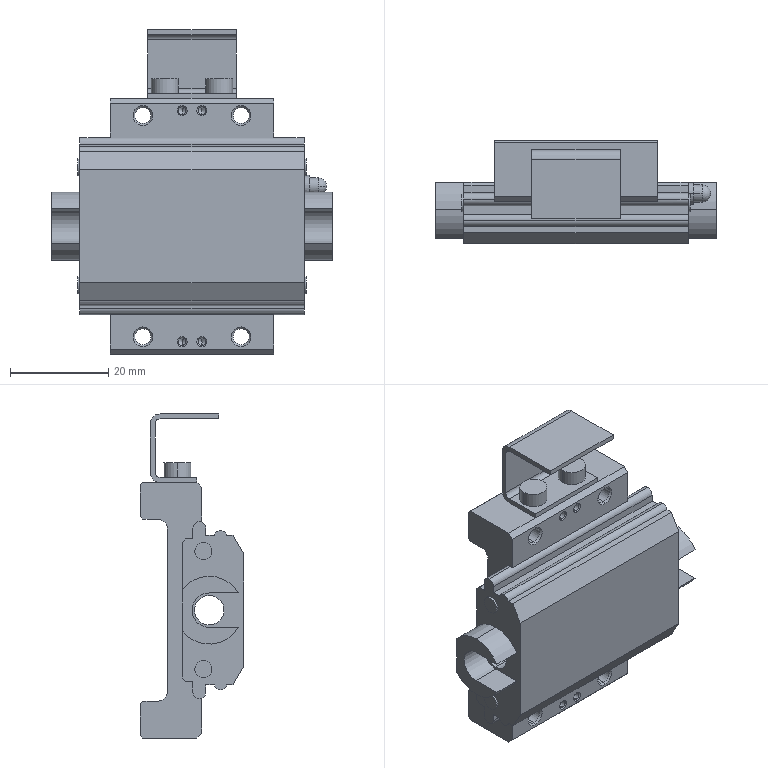Part | STEP file | QA-LX2005C_B1_200_EP3_bl | 1 solid | 194 faces | box 57 x 21 x 65.9 mm | volume 27894 mm3 | plane 75 | cylinder 69 | cone 48 | sphere 2 | commonest cylinder face diameters 3.5 x10 1.567 x8 2.459 x8 3.242 x8 2.6 x7 13.8 x6